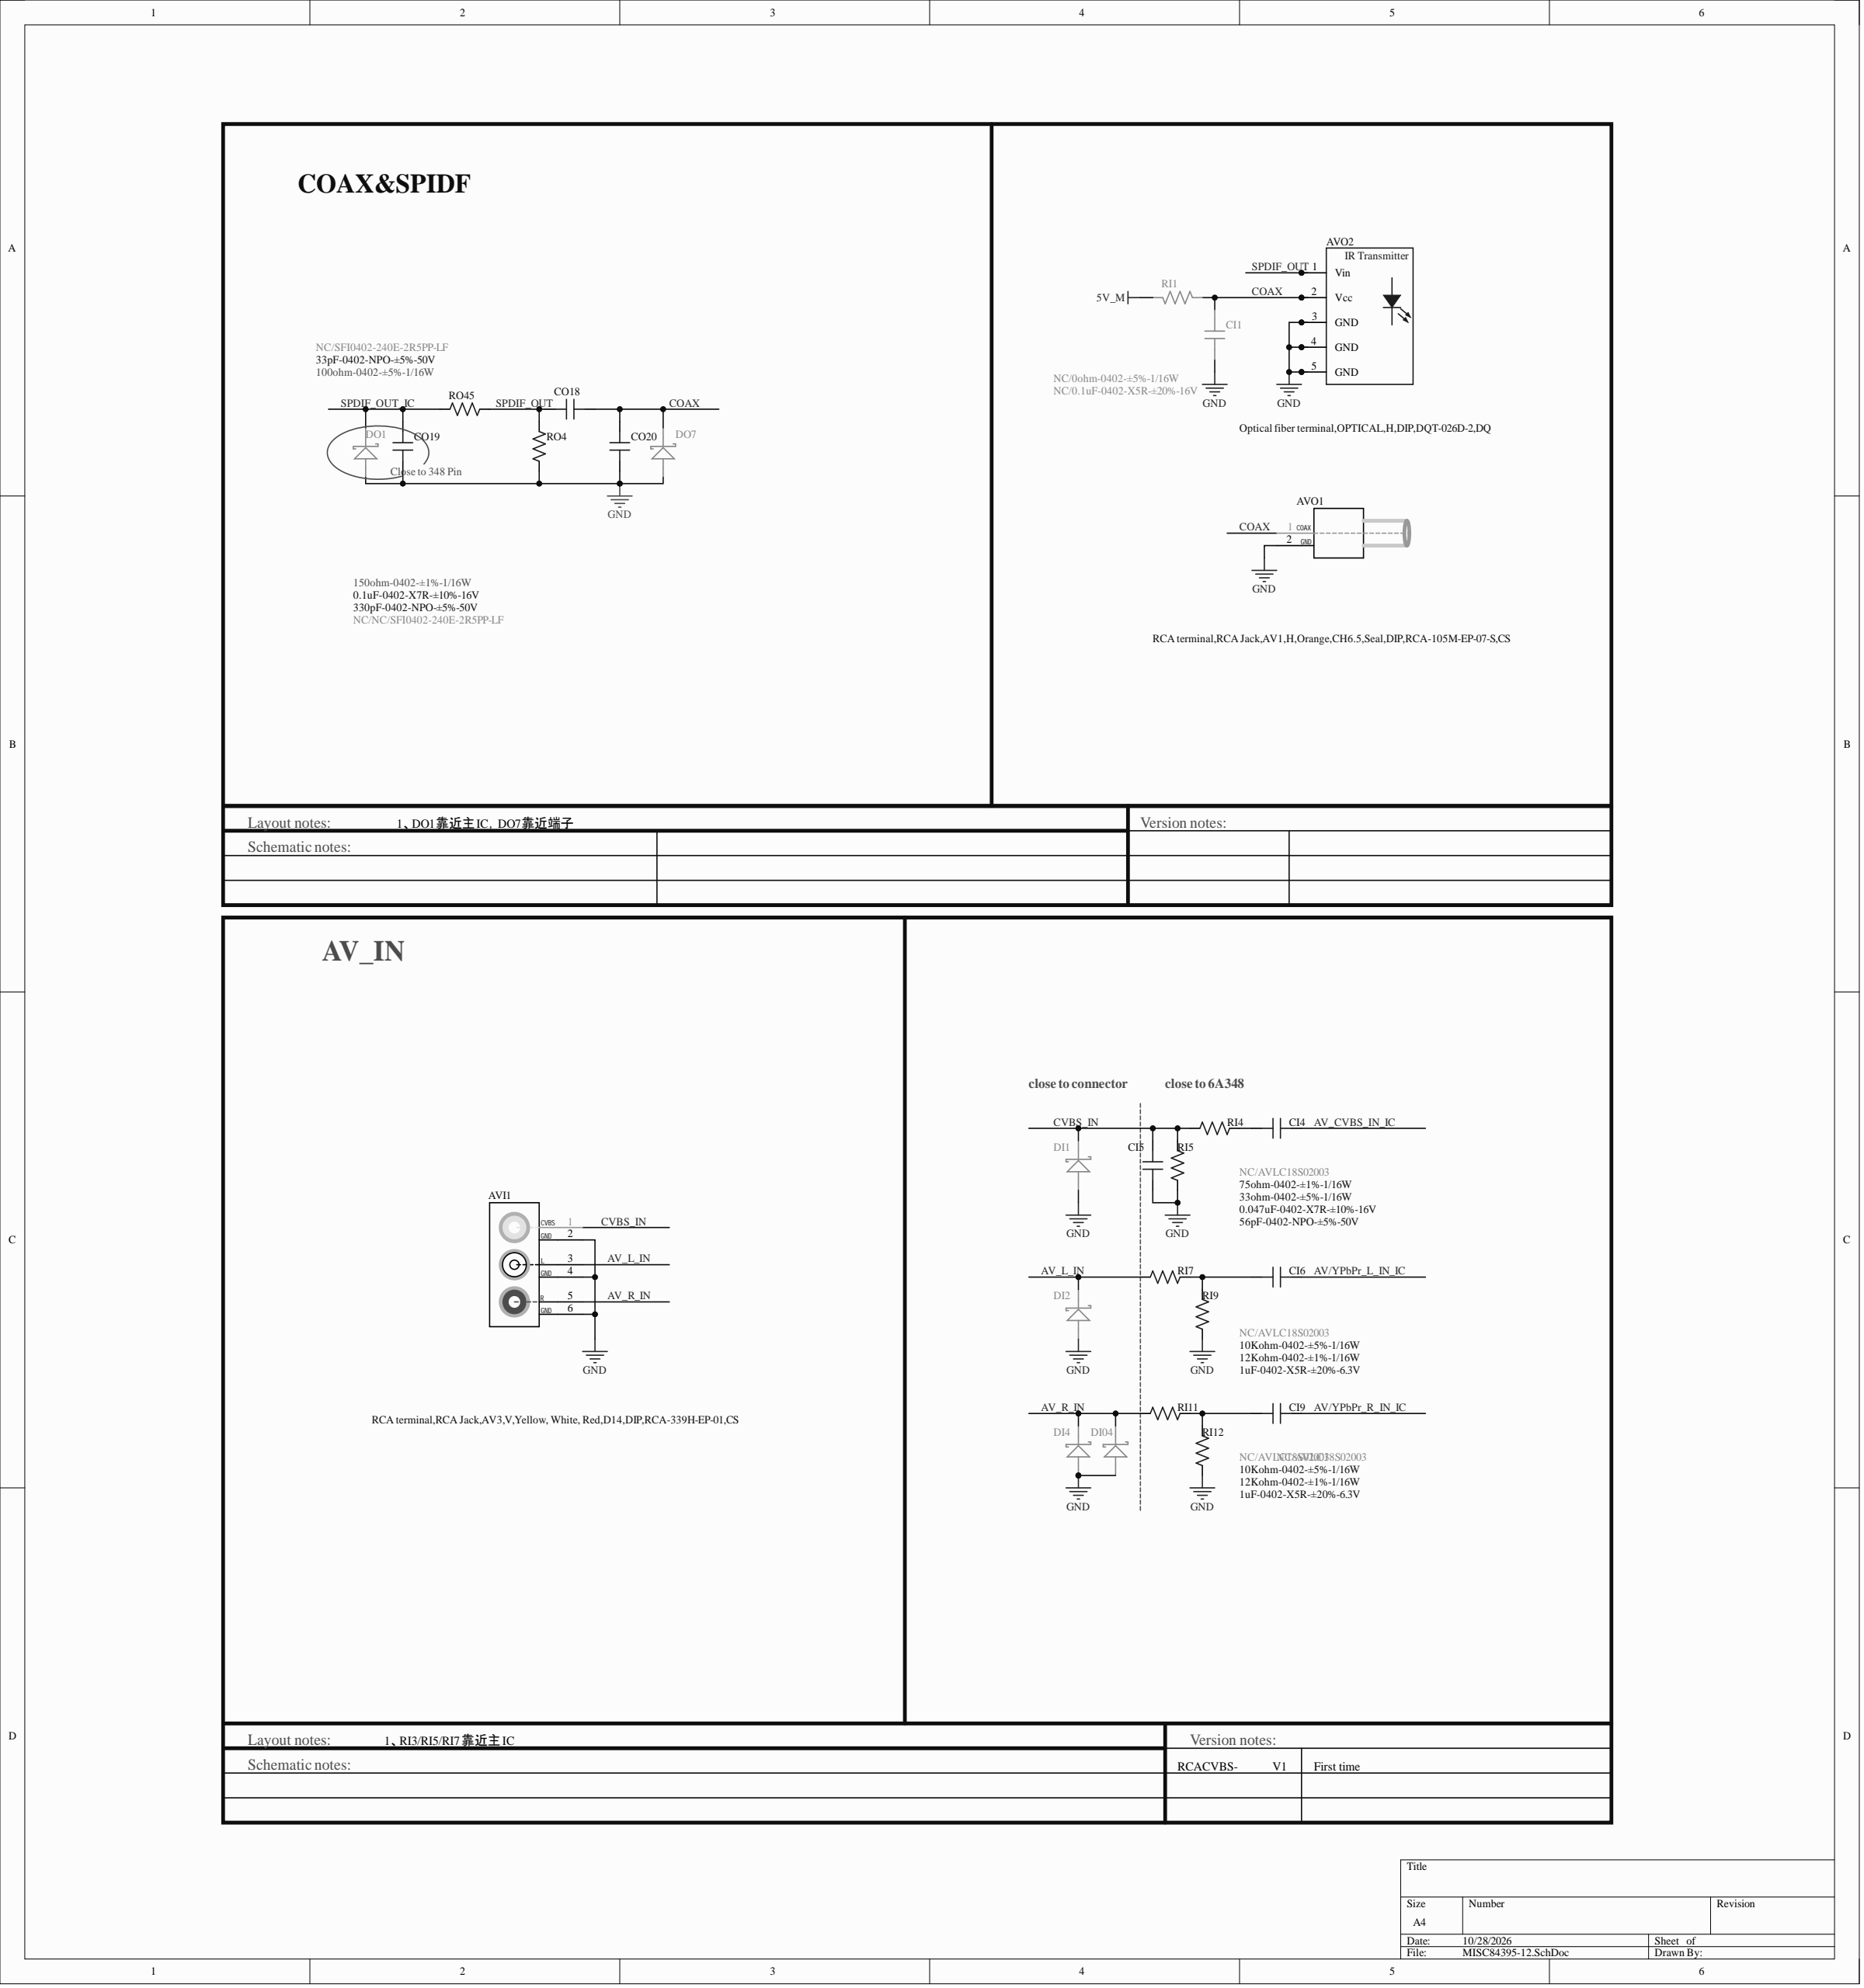Circuit board | Altium Designer | 951 parts | 509 nets | one sheet of the schematic
Parts on this sheet (reference | value | footprint):
AVI1 | RCA terminal,RCA Jack,AV3,V,Yellow, White, Red,D14,DIP,RCA-339H-EP-01,CS | AV3-V14-1
AVO1 | RCA terminal,RCA Jack,AV1,H,Orange,CH6.5,Seal,DIP,RCA-105M-EP-07-S,CS | AV1-H-1
AVO2 | Optical fiber terminal,OPTICAL,H,DIP,DQT-026D-2,DQ | OPTICAL-HD-3
CI1 | NC/0.1uF-0402-X5R-±20%-16V | C0402
CI4 | 0.047uF-0402-X7R-±10%-16V | C0402
CI5 | 56pF-0402-NPO-±5%-50V | C0402
CI6 | 1uF-0402-X5R-±20%-6.3V | C0402
CI9 | 1uF-0402-X5R-±20%-6.3V | C0402
CO18 | 0.1uF-0402-X7R-±10%-16V | C0402
CO19 | 33pF-0402-NPO-±5%-50V | C0402
CO20 | 330pF-0402-NPO-±5%-50V | C0402
DI1 | NC/AVLC18S02003 | DIODE-S0402
DI2 | NC/AVLC18S02003 | DIODE-S0402
DI4 | NC/AVLC18S02003 | DIODE-S0402
DI04 | NC/AVLC18S02003 | DIODE-S0402
DO1 | NC/NC/SFI0402-240E-2R5PP-LF | DIODE-S0402
DO7 | NC/SFI0402-240E-2R5PP-LF | DIODE-S0402
RI1 | NC/0ohm-0402-±5%-1/16W | R0402
RI4 | 33ohm-0402-±5%-1/16W | R0402
RI5 | 75ohm-0402-±1%-1/16W | R0402
RI7 | 10Kohm-0402-±5%-1/16W | R0402
RI9 | 12Kohm-0402-±1%-1/16W | R0402
RI11 | 10Kohm-0402-±5%-1/16W | R0402
RI12 | 12Kohm-0402-±1%-1/16W | R0402
RO4 | 150ohm-0402-±1%-1/16W | R0402
RO45 | 100ohm-0402-±5%-1/16W | R0402
Nets of these parts (net: part-pin ...):
SPDIF_OUT_IC: CO19-2 DO1-K RO45-1
SPDIF_OUT: AVO2-1 CO18-1 RO4-2 RO45-2
NetCI9_1: CI9-1 RI11-1 RI12-1
NetCI6_1: CI6-1 RI7-1 RI9-1
NetCI4_2: CI4-2 RI4-1
GND: AVI1-2 AVI1-4 AVI1-6 AVO1-2 AVO2-3 AVO2-4 AVO2-5 CI1-1 CI5-1 CO19-1 CO20-1 DI1-A DI2-A DI4-A DI04-A DO1-A DO7-A RI5-1 RI9-2 RI12-2 RO4-1
CVBS_IN: AVI1-1 CI5-2 DI1-K RI4-2 RI5-2
COAX: AVO1-1 AVO2-2 CI1-2 CO18-2 CO20-2 DO7-K RI1-2
AV_R_IN: AVI1-5 DI04-K DI4-K RI11-2
AV_L_IN: AVI1-3 DI2-K RI7-2
AV_CVBS_IN_IC: CI4-1
AV/YPbPr_R_IN_IC: CI9-2
AV/YPbPr_L_IN_IC: CI6-2
5V_M: RI1-1